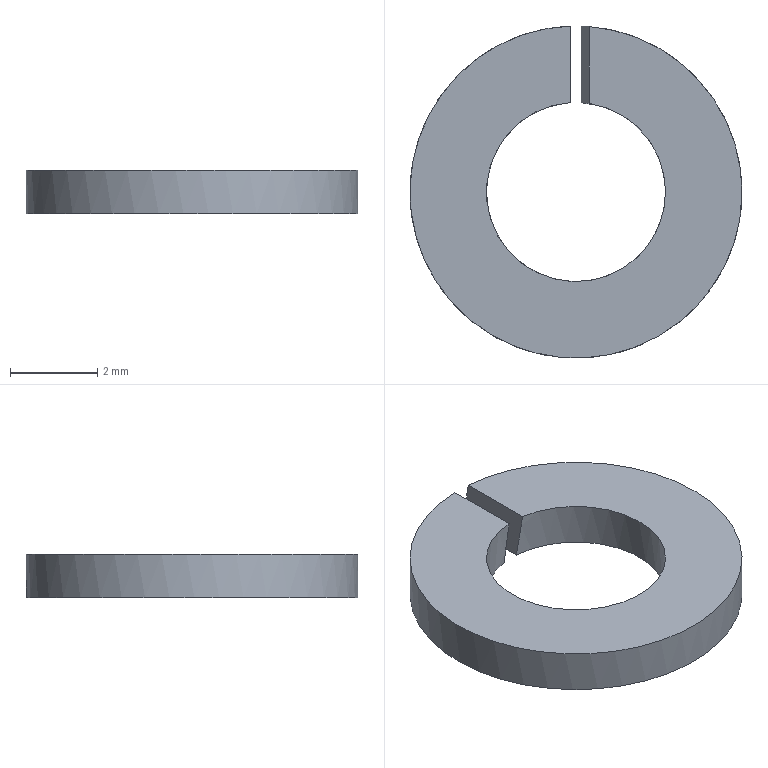Part | NX | features 5003_307_SLW4 2 | 1 solid | 6 faces | box 7.6 x 7.598 x 1 mm | volume 31.426 mm3 | plane 4 | cylinder 2 | commonest cylinder face diameters 4.1 x1 7.6 x1
STEP:
#1=CARTESIAN_POINT('',(216.945,70.198,-136.18));
#2=VERTEX_POINT('',#1);
#3=CARTESIAN_POINT('',(216.945,68.446,-136.18));
#4=VERTEX_POINT('',#3);
#5=CARTESIAN_POINT('',(216.945,70.2,-136.18));
#6=DIRECTION('',(0.,-1.,0.));
#7=VECTOR('',#6,1000.);
#8=LINE('',#5,#7);
#9=EDGE_CURVE('',#2,#4,#8,.T.);
#10=ORIENTED_EDGE('',*,*,#9,.F.);
#11=CARTESIAN_POINT('',(216.525,70.188,-136.18));
#12=VERTEX_POINT('',#11);
#13=CARTESIAN_POINT('',(216.825,66.4,-136.18));
#14=DIRECTION('',(0.,0.,-1.));
#15=DIRECTION('',(0.,1.,0.));
#16=AXIS2_PLACEMENT_3D('',#13,#14,#15);
#17=CIRCLE('',#16,3.8);
#18=EDGE_CURVE('',#2,#12,#17,.T.);
#19=ORIENTED_EDGE('',*,*,#18,.T.);
#20=CARTESIAN_POINT('',(216.525,68.428,-136.18));
#21=VERTEX_POINT('',#20);
#22=CARTESIAN_POINT('',(216.525,70.2,-136.18));
#23=DIRECTION('',(0.,-1.,0.));
#24=VECTOR('',#23,1000.);
#25=LINE('',#22,#24);
#26=EDGE_CURVE('',#12,#21,#25,.T.);
#27=ORIENTED_EDGE('',*,*,#26,.T.);
#28=CARTESIAN_POINT('',(216.825,66.4,-136.18));
#29=DIRECTION('',(0.,0.,-1.));
#30=DIRECTION('',(0.,1.,0.));
#31=AXIS2_PLACEMENT_3D('',#28,#29,#30);
#32=CIRCLE('',#31,2.05);
#33=EDGE_CURVE('',#4,#21,#32,.T.);
#34=ORIENTED_EDGE('',*,*,#33,.F.);
#35=EDGE_LOOP('',(#10,#19,#27,#34));
#36=FACE_BOUND('',#35,.T.);
#37=CARTESIAN_POINT('',(218.875,66.4,-136.18));
#38=DIRECTION('',(0.,0.,1.));
#39=DIRECTION('',(0.,-1.,0.));
#40=AXIS2_PLACEMENT_3D('',#37,#38,#39);
#41=PLANE('',#40);
#42=ADVANCED_FACE('',(#36),#41,.F.);
#43=CARTESIAN_POINT('',(217.125,70.188,-135.18));
#44=VERTEX_POINT('',#43);
#45=CARTESIAN_POINT('',(216.825,66.4,-136.847));
#46=DIRECTION('',(-0.9842,0.,0.1772));
#47=DIRECTION('',(-0.1772,0.,-0.9842));
#48=AXIS2_PLACEMENT_3D('',#45,#46,#47);
#49=ELLIPSE('',#48,21.45,3.8);
#50=EDGE_CURVE('',#44,#2,#49,.T.);
#51=ORIENTED_EDGE('',*,*,#50,.F.);
#52=CARTESIAN_POINT('',(216.705,70.198,-135.18));
#53=VERTEX_POINT('',#52);
#54=CARTESIAN_POINT('',(216.825,66.4,-135.18));
#55=DIRECTION('',(0.,0.,-1.));
#56=DIRECTION('',(0.,1.,0.));
#57=AXIS2_PLACEMENT_3D('',#54,#55,#56);
#58=CIRCLE('',#57,3.8);
#59=EDGE_CURVE('',#44,#53,#58,.T.);
#60=ORIENTED_EDGE('',*,*,#59,.T.);
#61=CARTESIAN_POINT('',(216.825,66.4,-134.513));
#62=DIRECTION('',(0.9842,0.,-0.1772));
#63=DIRECTION('',(-0.1772,0.,-0.9842));
#64=AXIS2_PLACEMENT_3D('',#61,#62,#63);
#65=ELLIPSE('',#64,21.45,3.8);
#66=EDGE_CURVE('',#12,#53,#65,.T.);
#67=ORIENTED_EDGE('',*,*,#66,.F.);
#68=ORIENTED_EDGE('',*,*,#18,.F.);
#69=EDGE_LOOP('',(#51,#60,#67,#68));
#70=FACE_BOUND('',#69,.T.);
#71=CARTESIAN_POINT('',(216.825,66.4,-136.18));
#72=DIRECTION('',(0.,0.,-1.));
#73=DIRECTION('',(0.,1.,0.));
#74=AXIS2_PLACEMENT_3D('',#71,#72,#73);
#75=CYLINDRICAL_SURFACE('',#74,3.8);
#76=ADVANCED_FACE('',(#70),#75,.T.);
#77=CARTESIAN_POINT('',(217.125,68.428,-135.18));
#78=VERTEX_POINT('',#77);
#79=CARTESIAN_POINT('',(217.125,70.2,-135.18));
#80=DIRECTION('',(0.,-1.,0.));
#81=VECTOR('',#80,1000.);
#82=LINE('',#79,#81);
#83=EDGE_CURVE('',#44,#78,#82,.T.);
#84=ORIENTED_EDGE('',*,*,#83,.T.);
#85=CARTESIAN_POINT('',(216.705,68.446,-135.18));
#86=VERTEX_POINT('',#85);
#87=CARTESIAN_POINT('',(216.825,66.4,-135.18));
#88=DIRECTION('',(0.,0.,-1.));
#89=DIRECTION('',(0.,1.,0.));
#90=AXIS2_PLACEMENT_3D('',#87,#88,#89);
#91=CIRCLE('',#90,2.05);
#92=EDGE_CURVE('',#78,#86,#91,.T.);
#93=ORIENTED_EDGE('',*,*,#92,.T.);
#94=CARTESIAN_POINT('',(216.705,70.2,-135.18));
#95=DIRECTION('',(0.,-1.,0.));
#96=VECTOR('',#95,1000.);
#97=LINE('',#94,#96);
#98=EDGE_CURVE('',#53,#86,#97,.T.);
#99=ORIENTED_EDGE('',*,*,#98,.F.);
#100=ORIENTED_EDGE('',*,*,#59,.F.);
#101=EDGE_LOOP('',(#84,#93,#99,#100));
#102=FACE_BOUND('',#101,.T.);
#103=CARTESIAN_POINT('',(218.875,66.4,-135.18));
#104=DIRECTION('',(0.,0.,-1.));
#105=DIRECTION('',(0.,1.,0.));
#106=AXIS2_PLACEMENT_3D('',#103,#104,#105);
#107=PLANE('',#106);
#108=ADVANCED_FACE('',(#102),#107,.F.);
#109=CARTESIAN_POINT('',(216.825,66.4,-136.847));
#110=DIRECTION('',(-0.9842,0.,0.1772));
#111=DIRECTION('',(-0.1772,0.,-0.9842));
#112=AXIS2_PLACEMENT_3D('',#109,#110,#111);
#113=ELLIPSE('',#112,11.572,2.05);
#114=EDGE_CURVE('',#4,#78,#113,.F.);
#115=ORIENTED_EDGE('',*,*,#114,.F.);
#116=ORIENTED_EDGE('',*,*,#33,.T.);
#117=CARTESIAN_POINT('',(216.825,66.4,-134.513));
#118=DIRECTION('',(0.9842,0.,-0.1772));
#119=DIRECTION('',(-0.1772,0.,-0.9842));
#120=AXIS2_PLACEMENT_3D('',#117,#118,#119);
#121=ELLIPSE('',#120,11.572,2.05);
#122=EDGE_CURVE('',#86,#21,#121,.F.);
#123=ORIENTED_EDGE('',*,*,#122,.F.);
#124=ORIENTED_EDGE('',*,*,#92,.F.);
#125=EDGE_LOOP('',(#115,#116,#123,#124));
#126=FACE_BOUND('',#125,.T.);
#127=CARTESIAN_POINT('',(216.825,66.4,-136.18));
#128=DIRECTION('',(0.,0.,-1.));
#129=DIRECTION('',(0.,1.,0.));
#130=AXIS2_PLACEMENT_3D('',#127,#128,#129);
#131=CYLINDRICAL_SURFACE('',#130,2.05);
#132=ADVANCED_FACE('',(#126),#131,.F.);
#133=ORIENTED_EDGE('',*,*,#66,.T.);
#134=ORIENTED_EDGE('',*,*,#98,.T.);
#135=ORIENTED_EDGE('',*,*,#122,.T.);
#136=ORIENTED_EDGE('',*,*,#26,.F.);
#137=EDGE_LOOP('',(#133,#134,#135,#136));
#138=FACE_BOUND('',#137,.T.);
#139=CARTESIAN_POINT('',(216.525,70.2,-136.18));
#140=DIRECTION('',(0.9842,0.,-0.1772));
#141=DIRECTION('',(-0.1772,0.,-0.9842));
#142=AXIS2_PLACEMENT_3D('',#139,#140,#141);
#143=PLANE('',#142);
#144=ADVANCED_FACE('',(#138),#143,.T.);
#145=ORIENTED_EDGE('',*,*,#50,.T.);
#146=ORIENTED_EDGE('',*,*,#9,.T.);
#147=ORIENTED_EDGE('',*,*,#114,.T.);
#148=ORIENTED_EDGE('',*,*,#83,.F.);
#149=EDGE_LOOP('',(#145,#146,#147,#148));
#150=FACE_BOUND('',#149,.T.);
#151=CARTESIAN_POINT('',(217.125,70.2,-135.18));
#152=DIRECTION('',(-0.9842,0.,0.1772));
#153=DIRECTION('',(0.1772,0.,0.9842));
#154=AXIS2_PLACEMENT_3D('',#151,#152,#153);
#155=PLANE('',#154);
#156=ADVANCED_FACE('',(#150),#155,.T.);
#157=CLOSED_SHELL('',(#42,#76,#108,#132,#144,#156));
#158=MANIFOLD_SOLID_BREP('',#157);
#159=(LENGTH_UNIT()NAMED_UNIT(*)SI_UNIT(.MILLI.,.METRE.));
#160=UNCERTAINTY_MEASURE_WITH_UNIT(LENGTH_MEASURE(0.00001),#159,'','');
#161=(NAMED_UNIT(*)PLANE_ANGLE_UNIT()SI_UNIT($,.RADIAN.));
#162=(NAMED_UNIT(*)SI_UNIT($,.STERADIAN.)SOLID_ANGLE_UNIT());
#163=(GEOMETRIC_REPRESENTATION_CONTEXT(3)GLOBAL_UNCERTAINTY_ASSIGNED_CONTEXT((#160))GLOBAL_UNIT_ASSIGNED_CONTEXT((#159,#161,#162))REPRESENTATION_CONTEXT('',''));
#164=ADVANCED_BREP_SHAPE_REPRESENTATION('',(#158),#163);